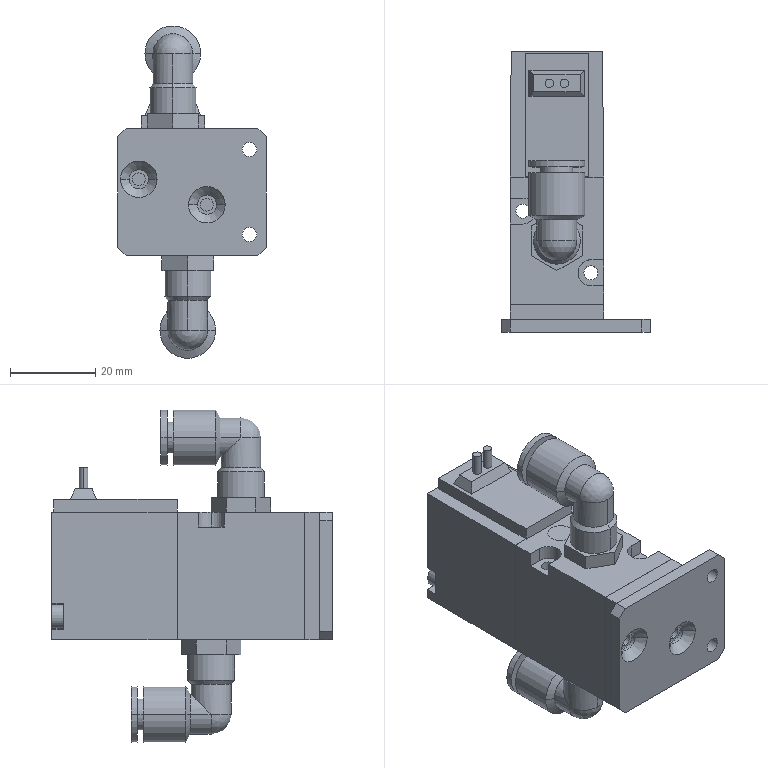Part | NX | features BREP 2 | 2 solids | 193 faces | box 35 x 66 x 78.15 mm | volume 39184 mm3 | plane 94 | cylinder 67 | cone 18 | spline 12 | sphere 2 | commonest cylinder face diameters 5.5 x8 9.35 x8 13.1 x8 2 x4 3 x4 3.3 x4